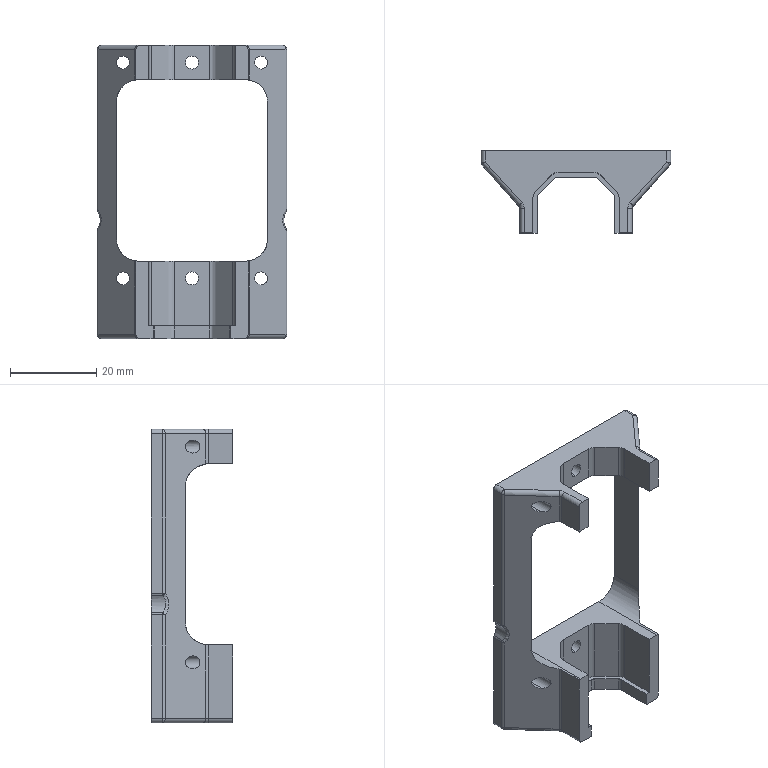Part | SolidWorks | features ICE 11, Fillet 7, MirrorPattern 3, Extrusion 1 | 1 solid | 105 faces | box 44 x 19 x 68 mm | volume 11985 mm3 | cylinder 54 | plane 37 | sphere 8 | torus 4 | spline 2 | commonest cylinder face diameters 2 x28 3 x12 4 x8 10 x4 7 x2